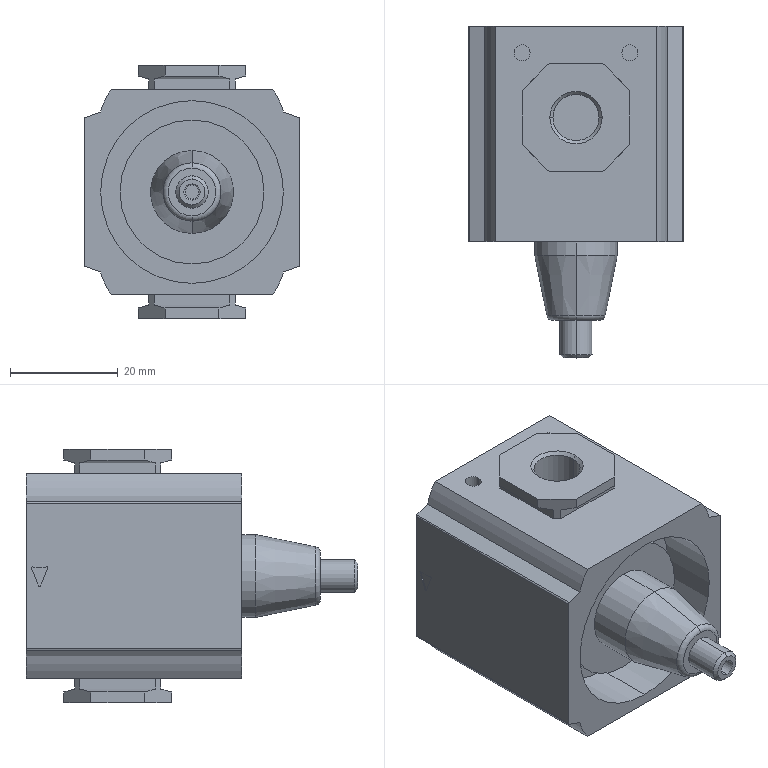Part | SolidWorks | features ICE 20, RefAxis 12, 3DProfileFeature 4, RevCut 3, Extrusion 1, Revolution 1 | 1 solid | 118 faces | box 40 x 61.6 x 47 mm | volume 55419 mm3 | plane 62 | cylinder 42 | cone 8 | torus 6 | commonest cylinder face diameters 3 x10 0.4 x7 0.6 x4 8.566 x4 24 x4 10 x3